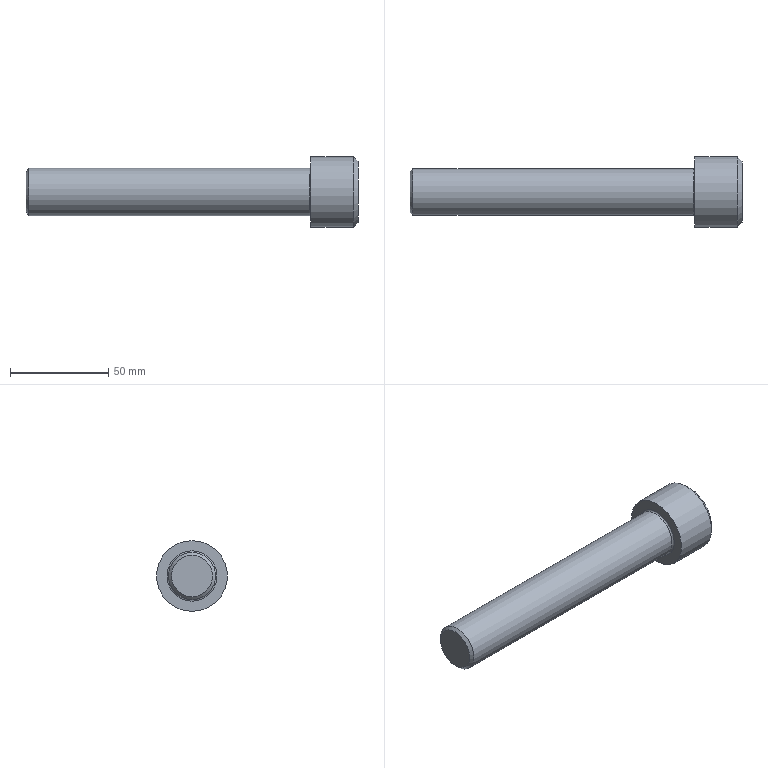Part | STEP file | solid 105 | 1 solid | 21 faces | box 169 x 36 x 36 mm | volume 85875 mm3 | plane 10 | sphere 6 | cylinder 2 | cone 2 | torus 1 | commonest cylinder face diameters 24 x1 36 x1